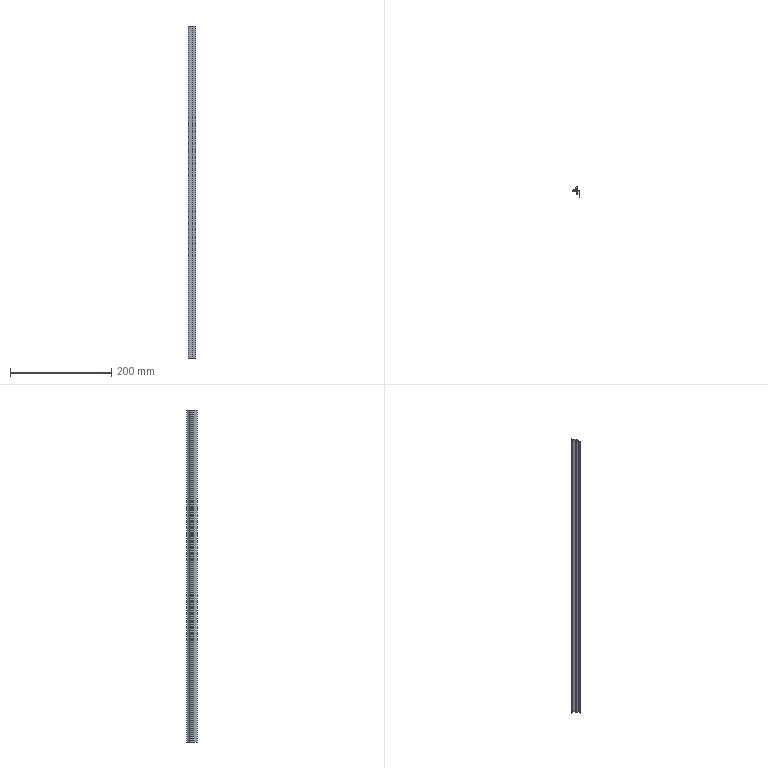Part | SolidWorks | features BaseBody 1, ICE 1, MoveFace 1 | 1 solid | 27 faces | box 14 x 20.3 x 657 mm | volume 33452 mm3 | plane 20 | cylinder 7 | commonest cylinder face diameters 0.387 x2 0.8 x2 0.4 x1 20 x1 22 x1
STEP:
#1=CARTESIAN_POINT('',(-5.304,-0.625,200.));
#2=VERTEX_POINT('',#1);
#3=CARTESIAN_POINT('',(-5.449,-0.8125,200.));
#4=VERTEX_POINT('',#3);
#5=CARTESIAN_POINT('',(-5.255,-0.8125,200.));
#6=DIRECTION('',(0.,0.,1.));
#7=DIRECTION('',(-1.,0.,0.));
#8=AXIS2_PLACEMENT_3D('',#5,#6,#7);
#9=CIRCLE('',#8,0.1937);
#10=EDGE_CURVE('',#2,#4,#9,.T.);
#11=ORIENTED_EDGE('',*,*,#10,.T.);
#12=CARTESIAN_POINT('',(-5.449,-0.8125,-457.));
#13=VERTEX_POINT('',#12);
#14=CARTESIAN_POINT('',(-5.449,-0.8125,230.));
#15=DIRECTION('',(0.,0.,-1.));
#16=VECTOR('',#15,1000.);
#17=LINE('',#14,#16);
#18=EDGE_CURVE('',#4,#13,#17,.T.);
#19=ORIENTED_EDGE('',*,*,#18,.T.);
#20=CARTESIAN_POINT('',(-5.304,-0.625,-457.));
#21=VERTEX_POINT('',#20);
#22=CARTESIAN_POINT('',(-5.255,-0.8125,-457.));
#23=DIRECTION('',(0.,0.,-1.));
#24=DIRECTION('',(1.,0.,0.));
#25=AXIS2_PLACEMENT_3D('',#22,#23,#24);
#26=CIRCLE('',#25,0.1937);
#27=EDGE_CURVE('',#13,#21,#26,.T.);
#28=ORIENTED_EDGE('',*,*,#27,.T.);
#29=CARTESIAN_POINT('',(-5.304,-0.625,230.));
#30=DIRECTION('',(0.,0.,-1.));
#31=VECTOR('',#30,1000.);
#32=LINE('',#29,#31);
#33=EDGE_CURVE('',#2,#21,#32,.T.);
#34=ORIENTED_EDGE('',*,*,#33,.F.);
#35=EDGE_LOOP('',(#11,#19,#28,#34));
#36=FACE_OUTER_BOUND('',#35,.T.);
#37=CARTESIAN_POINT('',(-5.255,-0.8125,230.));
#38=DIRECTION('',(0.,0.,-1.));
#39=DIRECTION('',(-1.,0.,0.));
#40=AXIS2_PLACEMENT_3D('',#37,#38,#39);
#41=CYLINDRICAL_SURFACE('',#40,0.1937);
#42=ADVANCED_FACE('',(#36),#41,.F.);
#43=CARTESIAN_POINT('',(5.,-1.,-457.));
#44=VERTEX_POINT('',#43);
#45=CARTESIAN_POINT('',(5.,-14.3,-457.));
#46=VERTEX_POINT('',#45);
#47=CARTESIAN_POINT('',(5.,29.623,-457.));
#48=DIRECTION('',(0.,-1.,0.));
#49=VECTOR('',#48,1000.);
#50=LINE('',#47,#49);
#51=EDGE_CURVE('',#44,#46,#50,.T.);
#52=ORIENTED_EDGE('',*,*,#51,.F.);
#53=CARTESIAN_POINT('',(5.,-1.,200.));
#54=VERTEX_POINT('',#53);
#55=CARTESIAN_POINT('',(5.,-1.,230.));
#56=DIRECTION('',(0.,0.,-1.));
#57=VECTOR('',#56,1000.);
#58=LINE('',#55,#57);
#59=EDGE_CURVE('',#54,#44,#58,.T.);
#60=ORIENTED_EDGE('',*,*,#59,.F.);
#61=CARTESIAN_POINT('',(5.,-14.3,200.));
#62=VERTEX_POINT('',#61);
#63=CARTESIAN_POINT('',(5.,-14.3,200.));
#64=DIRECTION('',(0.,1.,0.));
#65=VECTOR('',#64,1000.);
#66=LINE('',#63,#65);
#67=EDGE_CURVE('',#62,#54,#66,.T.);
#68=ORIENTED_EDGE('',*,*,#67,.F.);
#69=CARTESIAN_POINT('',(5.,-14.3,230.));
#70=DIRECTION('',(0.,0.,1.));
#71=VECTOR('',#70,1000.);
#72=LINE('',#69,#71);
#73=EDGE_CURVE('',#46,#62,#72,.T.);
#74=ORIENTED_EDGE('',*,*,#73,.F.);
#75=EDGE_LOOP('',(#52,#60,#68,#74));
#76=FACE_OUTER_BOUND('',#75,.T.);
#77=CARTESIAN_POINT('',(5.,-14.3,230.));
#78=DIRECTION('',(-1.,0.,0.));
#79=DIRECTION('',(0.,0.,1.));
#80=AXIS2_PLACEMENT_3D('',#77,#78,#79);
#81=PLANE('',#80);
#82=ADVANCED_FACE('',(#76),#81,.F.);
#83=CARTESIAN_POINT('',(-9.,-2.,-457.));
#84=VERTEX_POINT('',#83);
#85=CARTESIAN_POINT('',(-9.,-2.,200.));
#86=VERTEX_POINT('',#85);
#87=CARTESIAN_POINT('',(-9.,-2.,230.));
#88=DIRECTION('',(0.,0.,1.));
#89=VECTOR('',#88,1000.);
#90=LINE('',#87,#89);
#91=EDGE_CURVE('',#84,#86,#90,.T.);
#92=ORIENTED_EDGE('',*,*,#91,.F.);
#93=CARTESIAN_POINT('',(0.9,-2.,-457.));
#94=VERTEX_POINT('',#93);
#95=CARTESIAN_POINT('',(5.,-2.,-457.));
#96=DIRECTION('',(-1.,0.,0.));
#97=VECTOR('',#96,1000.);
#98=LINE('',#95,#97);
#99=EDGE_CURVE('',#94,#84,#98,.T.);
#100=ORIENTED_EDGE('',*,*,#99,.F.);
#101=CARTESIAN_POINT('',(0.9,-2.,200.));
#102=VERTEX_POINT('',#101);
#103=CARTESIAN_POINT('',(0.9,-2.,230.));
#104=DIRECTION('',(0.,0.,-1.));
#105=VECTOR('',#104,1000.);
#106=LINE('',#103,#105);
#107=EDGE_CURVE('',#102,#94,#106,.T.);
#108=ORIENTED_EDGE('',*,*,#107,.F.);
#109=CARTESIAN_POINT('',(5.,-2.,200.));
#110=DIRECTION('',(1.,0.,0.));
#111=VECTOR('',#110,1000.);
#112=LINE('',#109,#111);
#113=EDGE_CURVE('',#86,#102,#112,.T.);
#114=ORIENTED_EDGE('',*,*,#113,.F.);
#115=EDGE_LOOP('',(#92,#100,#108,#114));
#116=FACE_OUTER_BOUND('',#115,.T.);
#117=CARTESIAN_POINT('',(-9.,-2.,230.));
#118=DIRECTION('',(0.,1.,0.));
#119=DIRECTION('',(0.,0.,1.));
#120=AXIS2_PLACEMENT_3D('',#117,#118,#119);
#121=PLANE('',#120);
#122=ADVANCED_FACE('',(#116),#121,.F.);
#123=CARTESIAN_POINT('',(4.,-6.,200.));
#124=VERTEX_POINT('',#123);
#125=CARTESIAN_POINT('',(4.,-3.,200.));
#126=VERTEX_POINT('',#125);
#127=CARTESIAN_POINT('',(4.,29.623,200.));
#128=DIRECTION('',(0.,1.,0.));
#129=VECTOR('',#128,1000.);
#130=LINE('',#127,#129);
#131=EDGE_CURVE('',#124,#126,#130,.T.);
#132=ORIENTED_EDGE('',*,*,#131,.F.);
#133=CARTESIAN_POINT('',(1.,-6.,200.));
#134=VERTEX_POINT('',#133);
#135=CARTESIAN_POINT('',(5.,-6.,200.));
#136=DIRECTION('',(1.,0.,0.));
#137=VECTOR('',#136,1000.);
#138=LINE('',#135,#137);
#139=EDGE_CURVE('',#134,#124,#138,.T.);
#140=ORIENTED_EDGE('',*,*,#139,.F.);
#141=CARTESIAN_POINT('',(1.,-6.7,200.));
#142=VERTEX_POINT('',#141);
#143=CARTESIAN_POINT('',(1.,-6.,200.));
#144=DIRECTION('',(0.,-1.,0.));
#145=VECTOR('',#144,1000.);
#146=LINE('',#143,#145);
#147=EDGE_CURVE('',#134,#142,#146,.T.);
#148=ORIENTED_EDGE('',*,*,#147,.T.);
#149=CARTESIAN_POINT('',(-1.7,-6.7,200.));
#150=VERTEX_POINT('',#149);
#151=CARTESIAN_POINT('',(5.,-6.7,200.));
#152=DIRECTION('',(1.,0.,0.));
#153=VECTOR('',#152,1000.);
#154=LINE('',#151,#153);
#155=EDGE_CURVE('',#150,#142,#154,.T.);
#156=ORIENTED_EDGE('',*,*,#155,.F.);
#157=CARTESIAN_POINT('',(-1.7,-7.7,200.));
#158=VERTEX_POINT('',#157);
#159=CARTESIAN_POINT('',(-1.7,-6.7,200.));
#160=DIRECTION('',(0.,-1.,0.));
#161=VECTOR('',#160,1000.);
#162=LINE('',#159,#161);
#163=EDGE_CURVE('',#150,#158,#162,.T.);
#164=ORIENTED_EDGE('',*,*,#163,.T.);
#165=CARTESIAN_POINT('',(4.,-7.7,200.));
#166=VERTEX_POINT('',#165);
#167=CARTESIAN_POINT('',(5.,-7.7,200.));
#168=DIRECTION('',(-1.,0.,0.));
#169=VECTOR('',#168,1000.);
#170=LINE('',#167,#169);
#171=EDGE_CURVE('',#166,#158,#170,.T.);
#172=ORIENTED_EDGE('',*,*,#171,.F.);
#173=CARTESIAN_POINT('',(4.,-14.3,200.));
#174=VERTEX_POINT('',#173);
#175=CARTESIAN_POINT('',(4.,29.623,200.));
#176=DIRECTION('',(0.,1.,0.));
#177=VECTOR('',#176,1000.);
#178=LINE('',#175,#177);
#179=EDGE_CURVE('',#174,#166,#178,.T.);
#180=ORIENTED_EDGE('',*,*,#179,.F.);
#181=CARTESIAN_POINT('',(5.,-14.3,200.));
#182=DIRECTION('',(-1.,0.,0.));
#183=VECTOR('',#182,1000.);
#184=LINE('',#181,#183);
#185=EDGE_CURVE('',#62,#174,#184,.T.);
#186=ORIENTED_EDGE('',*,*,#185,.F.);
#187=ORIENTED_EDGE('',*,*,#67,.T.);
#188=CARTESIAN_POINT('',(-5.207,-1.,200.));
#189=VERTEX_POINT('',#188);
#190=CARTESIAN_POINT('',(5.,-1.,200.));
#191=DIRECTION('',(1.,0.,0.));
#192=VECTOR('',#191,1000.);
#193=LINE('',#190,#192);
#194=EDGE_CURVE('',#189,#54,#193,.T.);
#195=ORIENTED_EDGE('',*,*,#194,.F.);
#196=CARTESIAN_POINT('',(-5.255,-0.8125,200.));
#197=DIRECTION('',(0.,0.,1.));
#198=DIRECTION('',(-1.,0.,0.));
#199=AXIS2_PLACEMENT_3D('',#196,#197,#198);
#200=CIRCLE('',#199,0.1937);
#201=EDGE_CURVE('',#4,#189,#200,.T.);
#202=ORIENTED_EDGE('',*,*,#201,.F.);
#203=ORIENTED_EDGE('',*,*,#10,.F.);
#204=CARTESIAN_POINT('',(-1.368,3.063,200.));
#205=VERTEX_POINT('',#204);
#206=CARTESIAN_POINT('',(-10.628,9.,200.));
#207=DIRECTION('',(0.,0.,1.));
#208=DIRECTION('',(-1.,0.,0.));
#209=AXIS2_PLACEMENT_3D('',#206,#207,#208);
#210=CIRCLE('',#209,11.);
#211=EDGE_CURVE('',#2,#205,#210,.T.);
#212=ORIENTED_EDGE('',*,*,#211,.T.);
#213=CARTESIAN_POINT('',(-1.,2.955,200.));
#214=VERTEX_POINT('',#213);
#215=CARTESIAN_POINT('',(-1.2,2.955,200.));
#216=DIRECTION('',(0.,0.,1.));
#217=DIRECTION('',(-1.,0.,0.));
#218=AXIS2_PLACEMENT_3D('',#215,#216,#217);
#219=CIRCLE('',#218,0.2);
#220=EDGE_CURVE('',#214,#205,#219,.T.);
#221=ORIENTED_EDGE('',*,*,#220,.F.);
#222=CARTESIAN_POINT('',(-1.,1.5,200.));
#223=VERTEX_POINT('',#222);
#224=CARTESIAN_POINT('',(-1.,2.955,200.));
#225=DIRECTION('',(0.,1.,0.));
#226=VECTOR('',#225,1000.);
#227=LINE('',#224,#226);
#228=EDGE_CURVE('',#223,#214,#227,.T.);
#229=ORIENTED_EDGE('',*,*,#228,.F.);
#230=CARTESIAN_POINT('',(0.,1.5,200.));
#231=VERTEX_POINT('',#230);
#232=CARTESIAN_POINT('',(-1.,1.5,200.));
#233=DIRECTION('',(-1.,0.,0.));
#234=VECTOR('',#233,1000.);
#235=LINE('',#232,#234);
#236=EDGE_CURVE('',#231,#223,#235,.T.);
#237=ORIENTED_EDGE('',*,*,#236,.F.);
#238=CARTESIAN_POINT('',(0.,6.,200.));
#239=VERTEX_POINT('',#238);
#240=CARTESIAN_POINT('',(0.,1.5,200.));
#241=DIRECTION('',(0.,-1.,0.));
#242=VECTOR('',#241,1000.);
#243=LINE('',#240,#242);
#244=EDGE_CURVE('',#239,#231,#243,.T.);
#245=ORIENTED_EDGE('',*,*,#244,.F.);
#246=CARTESIAN_POINT('',(-0.8,6.,200.));
#247=VERTEX_POINT('',#246);
#248=CARTESIAN_POINT('',(0.,6.,200.));
#249=DIRECTION('',(1.,0.,0.));
#250=VECTOR('',#249,1000.);
#251=LINE('',#248,#250);
#252=EDGE_CURVE('',#247,#239,#251,.T.);
#253=ORIENTED_EDGE('',*,*,#252,.F.);
#254=CARTESIAN_POINT('',(-1.178,5.731,200.));
#255=VERTEX_POINT('',#254);
#256=CARTESIAN_POINT('',(-0.8,5.6,200.));
#257=DIRECTION('',(0.,0.,1.));
#258=DIRECTION('',(-1.,0.,0.));
#259=AXIS2_PLACEMENT_3D('',#256,#257,#258);
#260=CIRCLE('',#259,0.4);
#261=EDGE_CURVE('',#247,#255,#260,.T.);
#262=ORIENTED_EDGE('',*,*,#261,.T.);
#263=CARTESIAN_POINT('',(-8.678,-0.8077,200.));
#264=VERTEX_POINT('',#263);
#265=CARTESIAN_POINT('',(-10.628,9.,200.));
#266=DIRECTION('',(0.,0.,1.));
#267=DIRECTION('',(-1.,0.,0.));
#268=AXIS2_PLACEMENT_3D('',#265,#266,#267);
#269=CIRCLE('',#268,10.);
#270=EDGE_CURVE('',#264,#255,#269,.T.);
#271=ORIENTED_EDGE('',*,*,#270,.F.);
#272=CARTESIAN_POINT('',(-9.,-1.2,200.));
#273=VERTEX_POINT('',#272);
#274=CARTESIAN_POINT('',(-8.6,-1.2,200.));
#275=DIRECTION('',(0.,0.,1.));
#276=DIRECTION('',(-1.,0.,0.));
#277=AXIS2_PLACEMENT_3D('',#274,#275,#276);
#278=CIRCLE('',#277,0.4);
#279=EDGE_CURVE('',#264,#273,#278,.T.);
#280=ORIENTED_EDGE('',*,*,#279,.T.);
#281=CARTESIAN_POINT('',(-9.,8.,200.));
#282=DIRECTION('',(0.,-1.,0.));
#283=VECTOR('',#282,1000.);
#284=LINE('',#281,#283);
#285=EDGE_CURVE('',#273,#86,#284,.T.);
#286=ORIENTED_EDGE('',*,*,#285,.T.);
#287=ORIENTED_EDGE('',*,*,#113,.T.);
#288=CARTESIAN_POINT('',(0.9,-3.,200.));
#289=VERTEX_POINT('',#288);
#290=CARTESIAN_POINT('',(0.9,29.623,200.));
#291=DIRECTION('',(0.,1.,0.));
#292=VECTOR('',#291,1000.);
#293=LINE('',#290,#292);
#294=EDGE_CURVE('',#289,#102,#293,.T.);
#295=ORIENTED_EDGE('',*,*,#294,.F.);
#296=CARTESIAN_POINT('',(5.,-3.,200.));
#297=DIRECTION('',(-1.,0.,0.));
#298=VECTOR('',#297,1000.);
#299=LINE('',#296,#298);
#300=EDGE_CURVE('',#126,#289,#299,.T.);
#301=ORIENTED_EDGE('',*,*,#300,.F.);
#302=EDGE_LOOP('',(#132,#140,#148,#156,#164,#172,#180,#186,#187,#195,#202,#203,#212,#221,#229,#237,#245,#253,#262,#271,#280,#286,#287,#295,#301));
#303=FACE_OUTER_BOUND('',#302,.T.);
#304=CARTESIAN_POINT('',(5.,29.623,200.));
#305=DIRECTION('',(0.,0.,-1.));
#306=DIRECTION('',(-1.,0.,0.));
#307=AXIS2_PLACEMENT_3D('',#304,#305,#306);
#308=PLANE('',#307);
#309=ADVANCED_FACE('',(#303),#308,.F.);
#310=ORIENTED_EDGE('',*,*,#185,.T.);
#311=CARTESIAN_POINT('',(4.,-14.3,-457.));
#312=VERTEX_POINT('',#311);
#313=CARTESIAN_POINT('',(4.,-14.3,230.));
#314=DIRECTION('',(0.,0.,1.));
#315=VECTOR('',#314,1000.);
#316=LINE('',#313,#315);
#317=EDGE_CURVE('',#312,#174,#316,.T.);
#318=ORIENTED_EDGE('',*,*,#317,.F.);
#319=CARTESIAN_POINT('',(5.,-14.3,-457.));
#320=DIRECTION('',(-1.,0.,0.));
#321=VECTOR('',#320,1000.);
#322=LINE('',#319,#321);
#323=EDGE_CURVE('',#46,#312,#322,.T.);
#324=ORIENTED_EDGE('',*,*,#323,.F.);
#325=ORIENTED_EDGE('',*,*,#73,.T.);
#326=EDGE_LOOP('',(#310,#318,#324,#325));
#327=FACE_OUTER_BOUND('',#326,.T.);
#328=CARTESIAN_POINT('',(4.,-14.3,230.));
#329=DIRECTION('',(0.,1.,0.));
#330=DIRECTION('',(0.,0.,1.));
#331=AXIS2_PLACEMENT_3D('',#328,#329,#330);
#332=PLANE('',#331);
#333=ADVANCED_FACE('',(#327),#332,.F.);
#334=ORIENTED_EDGE('',*,*,#51,.T.);
#335=ORIENTED_EDGE('',*,*,#323,.T.);
#336=CARTESIAN_POINT('',(4.,-7.7,-457.));
#337=VERTEX_POINT('',#336);
#338=CARTESIAN_POINT('',(4.,-7.7,-457.));
#339=DIRECTION('',(0.,-1.,0.));
#340=VECTOR('',#339,1000.);
#341=LINE('',#338,#340);
#342=EDGE_CURVE('',#337,#312,#341,.T.);
#343=ORIENTED_EDGE('',*,*,#342,.F.);
#344=CARTESIAN_POINT('',(-1.7,-7.7,-457.));
#345=VERTEX_POINT('',#344);
#346=CARTESIAN_POINT('',(-1.7,-7.7,-457.));
#347=DIRECTION('',(1.,0.,0.));
#348=VECTOR('',#347,1000.);
#349=LINE('',#346,#348);
#350=EDGE_CURVE('',#345,#337,#349,.T.);
#351=ORIENTED_EDGE('',*,*,#350,.F.);
#352=CARTESIAN_POINT('',(-1.7,-6.7,-457.));
#353=VERTEX_POINT('',#352);
#354=CARTESIAN_POINT('',(-1.7,29.623,-457.));
#355=DIRECTION('',(0.,1.,0.));
#356=VECTOR('',#355,1000.);
#357=LINE('',#354,#356);
#358=EDGE_CURVE('',#345,#353,#357,.T.);
#359=ORIENTED_EDGE('',*,*,#358,.T.);
#360=CARTESIAN_POINT('',(1.,-6.7,-457.));
#361=VERTEX_POINT('',#360);
#362=CARTESIAN_POINT('',(1.,-6.7,-457.));
#363=DIRECTION('',(-1.,0.,0.));
#364=VECTOR('',#363,1000.);
#365=LINE('',#362,#364);
#366=EDGE_CURVE('',#361,#353,#365,.T.);
#367=ORIENTED_EDGE('',*,*,#366,.F.);
#368=CARTESIAN_POINT('',(1.,-6.,-457.));
#369=VERTEX_POINT('',#368);
#370=CARTESIAN_POINT('',(1.,29.623,-457.));
#371=DIRECTION('',(0.,1.,0.));
#372=VECTOR('',#371,1000.);
#373=LINE('',#370,#372);
#374=EDGE_CURVE('',#361,#369,#373,.T.);
#375=ORIENTED_EDGE('',*,*,#374,.T.);
#376=CARTESIAN_POINT('',(4.,-6.,-457.));
#377=VERTEX_POINT('',#376);
#378=CARTESIAN_POINT('',(4.,-6.,-457.));
#379=DIRECTION('',(-1.,0.,0.));
#380=VECTOR('',#379,1000.);
#381=LINE('',#378,#380);
#382=EDGE_CURVE('',#377,#369,#381,.T.);
#383=ORIENTED_EDGE('',*,*,#382,.F.);
#384=CARTESIAN_POINT('',(4.,-3.,-457.));
#385=VERTEX_POINT('',#384);
#386=CARTESIAN_POINT('',(4.,-3.,-457.));
#387=DIRECTION('',(0.,-1.,0.));
#388=VECTOR('',#387,1000.);
#389=LINE('',#386,#388);
#390=EDGE_CURVE('',#385,#377,#389,.T.);
#391=ORIENTED_EDGE('',*,*,#390,.F.);
#392=CARTESIAN_POINT('',(0.9,-3.,-457.));
#393=VERTEX_POINT('',#392);
#394=CARTESIAN_POINT('',(0.9,-3.,-457.));
#395=DIRECTION('',(1.,0.,0.));
#396=VECTOR('',#395,1000.);
#397=LINE('',#394,#396);
#398=EDGE_CURVE('',#393,#385,#397,.T.);
#399=ORIENTED_EDGE('',*,*,#398,.F.);
#400=CARTESIAN_POINT('',(0.9,-2.,-457.));
#401=DIRECTION('',(0.,-1.,0.));
#402=VECTOR('',#401,1000.);
#403=LINE('',#400,#402);
#404=EDGE_CURVE('',#94,#393,#403,.T.);
#405=ORIENTED_EDGE('',*,*,#404,.F.);
#406=ORIENTED_EDGE('',*,*,#99,.T.);
#407=CARTESIAN_POINT('',(-9.,-1.2,-457.));
#408=VERTEX_POINT('',#407);
#409=CARTESIAN_POINT('',(-9.,-1.2,-457.));
#410=DIRECTION('',(0.,-1.,0.));
#411=VECTOR('',#410,1000.);
#412=LINE('',#409,#411);
#413=EDGE_CURVE('',#408,#84,#412,.T.);
#414=ORIENTED_EDGE('',*,*,#413,.F.);
#415=CARTESIAN_POINT('',(-8.678,-0.8077,-457.));
#416=VERTEX_POINT('',#415);
#417=CARTESIAN_POINT('',(-8.6,-1.2,-457.));
#418=DIRECTION('',(0.,0.,-1.));
#419=DIRECTION('',(1.,0.,0.));
#420=AXIS2_PLACEMENT_3D('',#417,#418,#419);
#421=CIRCLE('',#420,0.4);
#422=EDGE_CURVE('',#408,#416,#421,.T.);
#423=ORIENTED_EDGE('',*,*,#422,.T.);
#424=CARTESIAN_POINT('',(-1.178,5.731,-457.));
#425=VERTEX_POINT('',#424);
#426=CARTESIAN_POINT('',(-10.628,9.,-457.));
#427=DIRECTION('',(0.,0.,-1.));
#428=DIRECTION('',(1.,0.,0.));
#429=AXIS2_PLACEMENT_3D('',#426,#427,#428);
#430=CIRCLE('',#429,10.);
#431=EDGE_CURVE('',#425,#416,#430,.T.);
#432=ORIENTED_EDGE('',*,*,#431,.F.);
#433=CARTESIAN_POINT('',(-0.8,6.,-457.));
#434=VERTEX_POINT('',#433);
#435=CARTESIAN_POINT('',(-0.8,5.6,-457.));
#436=DIRECTION('',(0.,0.,-1.));
#437=DIRECTION('',(1.,0.,0.));
#438=AXIS2_PLACEMENT_3D('',#435,#436,#437);
#439=CIRCLE('',#438,0.4);
#440=EDGE_CURVE('',#425,#434,#439,.T.);
#441=ORIENTED_EDGE('',*,*,#440,.T.);
#442=CARTESIAN_POINT('',(0.,6.,-457.));
#443=VERTEX_POINT('',#442);
#444=CARTESIAN_POINT('',(0.,6.,-457.));
#445=DIRECTION('',(-1.,0.,0.));
#446=VECTOR('',#445,1000.);
#447=LINE('',#444,#446);
#448=EDGE_CURVE('',#443,#434,#447,.T.);
#449=ORIENTED_EDGE('',*,*,#448,.F.);
#450=CARTESIAN_POINT('',(0.,1.5,-457.));
#451=VERTEX_POINT('',#450);
#452=CARTESIAN_POINT('',(0.,1.5,-457.));
#453=DIRECTION('',(0.,1.,0.));
#454=VECTOR('',#453,1000.);
#455=LINE('',#452,#454);
#456=EDGE_CURVE('',#451,#443,#455,.T.);
#457=ORIENTED_EDGE('',*,*,#456,.F.);
#458=CARTESIAN_POINT('',(-1.,1.5,-457.));
#459=VERTEX_POINT('',#458);
#460=CARTESIAN_POINT('',(-1.,1.5,-457.));
#461=DIRECTION('',(1.,0.,0.));
#462=VECTOR('',#461,1000.);
#463=LINE('',#460,#462);
#464=EDGE_CURVE('',#459,#451,#463,.T.);
#465=ORIENTED_EDGE('',*,*,#464,.F.);
#466=CARTESIAN_POINT('',(-1.,2.955,-457.));
#467=VERTEX_POINT('',#466);
#468=CARTESIAN_POINT('',(-1.,2.955,-457.));
#469=DIRECTION('',(0.,-1.,0.));
#470=VECTOR('',#469,1000.);
#471=LINE('',#468,#470);
#472=EDGE_CURVE('',#467,#459,#471,.T.);
#473=ORIENTED_EDGE('',*,*,#472,.F.);
#474=CARTESIAN_POINT('',(-1.368,3.063,-457.));
#475=VERTEX_POINT('',#474);
#476=CARTESIAN_POINT('',(-1.2,2.955,-457.));
#477=DIRECTION('',(0.,0.,-1.));
#478=DIRECTION('',(1.,0.,0.));
#479=AXIS2_PLACEMENT_3D('',#476,#477,#478);
#480=CIRCLE('',#479,0.2);
#481=EDGE_CURVE('',#475,#467,#480,.T.);
#482=ORIENTED_EDGE('',*,*,#481,.F.);
#483=CARTESIAN_POINT('',(-10.628,9.,-457.));
#484=DIRECTION('',(0.,0.,-1.));
#485=DIRECTION('',(1.,0.,0.));
#486=AXIS2_PLACEMENT_3D('',#483,#484,#485);
#487=CIRCLE('',#486,11.);
#488=EDGE_CURVE('',#475,#21,#487,.T.);
#489=ORIENTED_EDGE('',*,*,#488,.T.);
#490=ORIENTED_EDGE('',*,*,#27,.F.);
#491=CARTESIAN_POINT('',(-5.207,-1.,-457.));
#492=VERTEX_POINT('',#491);
#493=CARTESIAN_POINT('',(-5.255,-0.8125,-457.));
#494=DIRECTION('',(0.,0.,-1.));
#495=DIRECTION('',(1.,0.,0.));
#496=AXIS2_PLACEMENT_3D('',#493,#494,#495);
#497=CIRCLE('',#496,0.1937);
#498=EDGE_CURVE('',#492,#13,#497,.T.);
#499=ORIENTED_EDGE('',*,*,#498,.F.);
#500=CARTESIAN_POINT('',(5.,-1.,-457.));
#501=DIRECTION('',(-1.,0.,0.));
#502=VECTOR('',#501,1000.);
#503=LINE('',#500,#502);
#504=EDGE_CURVE('',#44,#492,#503,.T.);
#505=ORIENTED_EDGE('',*,*,#504,.F.);
#506=EDGE_LOOP('',(#334,#335,#343,#351,#359,#367,#375,#383,#391,#399,#405,#406,#414,#423,#432,#441,#449,#457,#465,#473,#482,#489,#490,#499,#505));
#507=FACE_OUTER_BOUND('',#506,.T.);
#508=CARTESIAN_POINT('',(5.,29.623,-457.));
#509=DIRECTION('',(0.,0.,1.));
#510=DIRECTION('',(1.,0.,0.));
#511=AXIS2_PLACEMENT_3D('',#508,#509,#510);
#512=PLANE('',#511);
#513=ADVANCED_FACE('',(#507),#512,.F.);
#514=ORIENTED_EDGE('',*,*,#59,.T.);
#515=ORIENTED_EDGE('',*,*,#504,.T.);
#516=CARTESIAN_POINT('',(-5.207,-1.,230.));
#517=DIRECTION('',(0.,0.,-1.));
#518=VECTOR('',#517,1000.);
#519=LINE('',#516,#518);
#520=EDGE_CURVE('',#189,#492,#519,.T.);
#521=ORIENTED_EDGE('',*,*,#520,.F.);
#522=ORIENTED_EDGE('',*,*,#194,.T.);
#523=EDGE_LOOP('',(#514,#515,#521,#522));
#524=FACE_OUTER_BOUND('',#523,.T.);
#525=CARTESIAN_POINT('',(5.,-1.,230.));
#526=DIRECTION('',(0.,-1.,0.));
#527=DIRECTION('',(0.,0.,-1.));
#528=AXIS2_PLACEMENT_3D('',#525,#526,#527);
#529=PLANE('',#528);
#530=ADVANCED_FACE('',(#524),#529,.F.);
#531=CARTESIAN_POINT('',(-9.,-1.2,230.));
#532=DIRECTION('',(0.,0.,1.));
#533=VECTOR('',#532,1000.);
#534=LINE('',#531,#533);
#535=EDGE_CURVE('',#408,#273,#534,.T.);
#536=ORIENTED_EDGE('',*,*,#535,.F.);
#537=ORIENTED_EDGE('',*,*,#413,.T.);
#538=ORIENTED_EDGE('',*,*,#91,.T.);
#539=ORIENTED_EDGE('',*,*,#285,.F.);
#540=EDGE_LOOP('',(#536,#537,#538,#539));
#541=FACE_OUTER_BOUND('',#540,.T.);
#542=CARTESIAN_POINT('',(-9.,-1.2,230.));
#543=DIRECTION('',(1.,0.,0.));
#544=DIRECTION('',(0.,0.,-1.));
#545=AXIS2_PLACEMENT_3D('',#542,#543,#544);
#546=PLANE('',#545);
#547=ADVANCED_FACE('',(#541),#546,.F.);
#548=ORIENTED_EDGE('',*,*,#294,.T.);
#549=ORIENTED_EDGE('',*,*,#107,.T.);
#550=ORIENTED_EDGE('',*,*,#404,.T.);
#551=CARTESIAN_POINT('',(0.9,-3.,230.));
#552=DIRECTION('',(0.,0.,-1.));
#553=VECTOR('',#552,1000.);
#554=LINE('',#551,#553);
#555=EDGE_CURVE('',#289,#393,#554,.T.);
#556=ORIENTED_EDGE('',*,*,#555,.F.);
#557=EDGE_LOOP('',(#548,#549,#550,#556));
#558=FACE_OUTER_BOUND('',#557,.T.);
#559=CARTESIAN_POINT('',(0.9,-2.,230.));
#560=DIRECTION('',(1.,0.,0.));
#561=DIRECTION('',(0.,0.,-1.));
#562=AXIS2_PLACEMENT_3D('',#559,#560,#561);
#563=PLANE('',#562);
#564=ADVANCED_FACE('',(#558),#563,.F.);
#565=ORIENTED_EDGE('',*,*,#300,.T.);
#566=ORIENTED_EDGE('',*,*,#555,.T.);
#567=ORIENTED_EDGE('',*,*,#398,.T.);
#568=CARTESIAN_POINT('',(4.,-3.,230.));
#569=DIRECTION('',(0.,0.,-1.));
#570=VECTOR('',#569,1000.);
#571=LINE('',#568,#570);
#572=EDGE_CURVE('',#126,#385,#571,.T.);
#573=ORIENTED_EDGE('',*,*,#572,.F.);
#574=EDGE_LOOP('',(#565,#566,#567,#573));
#575=FACE_OUTER_BOUND('',#574,.T.);
#576=CARTESIAN_POINT('',(0.9,-3.,230.));
#577=DIRECTION('',(0.,1.,0.));
#578=DIRECTION('',(0.,0.,1.));
#579=AXIS2_PLACEMENT_3D('',#576,#577,#578);
#580=PLANE('',#579);
#581=ADVANCED_FACE('',(#575),#580,.F.);
#582=ORIENTED_EDGE('',*,*,#131,.T.);
#583=ORIENTED_EDGE('',*,*,#572,.T.);
#584=ORIENTED_EDGE('',*,*,#390,.T.);
#585=CARTESIAN_POINT('',(4.,-6.,230.));
#586=DIRECTION('',(0.,0.,-1.));
#587=VECTOR('',#586,1000.);
#588=LINE('',#585,#587);
#589=EDGE_CURVE('',#124,#377,#588,.T.);
#590=ORIENTED_EDGE('',*,*,#589,.F.);
#591=EDGE_LOOP('',(#582,#583,#584,#590));
#592=FACE_OUTER_BOUND('',#591,.T.);
#593=CARTESIAN_POINT('',(4.,-3.,230.));
#594=DIRECTION('',(1.,0.,0.));
#595=DIRECTION('',(0.,0.,-1.));
#596=AXIS2_PLACEMENT_3D('',#593,#594,#595);
#597=PLANE('',#596);
#598=ADVANCED_FACE('',(#592),#597,.F.);
#599=ORIENTED_EDGE('',*,*,#139,.T.);
#600=ORIENTED_EDGE('',*,*,#589,.T.);
#601=ORIENTED_EDGE('',*,*,#382,.T.);
#602=CARTESIAN_POINT('',(1.,-6.,230.));
#603=DIRECTION('',(0.,0.,-1.));
#604=VECTOR('',#603,1000.);
#605=LINE('',#602,#604);
#606=EDGE_CURVE('',#134,#369,#605,.T.);
#607=ORIENTED_EDGE('',*,*,#606,.F.);
#608=EDGE_LOOP('',(#599,#600,#601,#607));
#609=FACE_OUTER_BOUND('',#608,.T.);
#610=CARTESIAN_POINT('',(4.,-6.,230.));
#611=DIRECTION('',(0.,-1.,0.));
#612=DIRECTION('',(0.,0.,-1.));
#613=AXIS2_PLACEMENT_3D('',#610,#611,#612);
#614=PLANE('',#613);
#615=ADVANCED_FACE('',(#609),#614,.F.);
#616=ORIENTED_EDGE('',*,*,#155,.T.);
#617=CARTESIAN_POINT('',(1.,-6.7,230.));
#618=DIRECTION('',(0.,0.,1.));
#619=VECTOR('',#618,1000.);
#620=LINE('',#617,#619);
#621=EDGE_CURVE('',#361,#142,#620,.T.);
#622=ORIENTED_EDGE('',*,*,#621,.F.);
#623=ORIENTED_EDGE('',*,*,#366,.T.);
#624=CARTESIAN_POINT('',(-1.7,-6.7,230.));
#625=DIRECTION('',(0.,0.,-1.));
#626=VECTOR('',#625,1000.);
#627=LINE('',#624,#626);
#628=EDGE_CURVE('',#150,#353,#627,.T.);
#629=ORIENTED_EDGE('',*,*,#628,.F.);
#630=EDGE_LOOP('',(#616,#622,#623,#629));
#631=FACE_OUTER_BOUND('',#630,.T.);
#632=CARTESIAN_POINT('',(1.,-6.7,230.));
#633=DIRECTION('',(0.,-1.,0.));
#634=DIRECTION('',(0.,0.,-1.));
#635=AXIS2_PLACEMENT_3D('',#632,#633,#634);
#636=PLANE('',#635);
#637=ADVANCED_FACE('',(#631),#636,.F.);
#638=ORIENTED_EDGE('',*,*,#171,.T.);
#639=CARTESIAN_POINT('',(-1.7,-7.7,230.));
#640=DIRECTION('',(0.,0.,1.));
#641=VECTOR('',#640,1000.);
#642=LINE('',#639,#641);
#643=EDGE_CURVE('',#345,#158,#642,.T.);
#644=ORIENTED_EDGE('',*,*,#643,.F.);
#645=ORIENTED_EDGE('',*,*,#350,.T.);
#646=CARTESIAN_POINT('',(4.,-7.7,230.));
#647=DIRECTION('',(0.,0.,-1.));
#648=VECTOR('',#647,1000.);
#649=LINE('',#646,#648);
#650=EDGE_CURVE('',#166,#337,#649,.T.);
#651=ORIENTED_EDGE('',*,*,#650,.F.);
#652=EDGE_LOOP('',(#638,#644,#645,#651));
#653=FACE_OUTER_BOUND('',#652,.T.);
#654=CARTESIAN_POINT('',(-1.7,-7.7,230.));
#655=DIRECTION('',(0.,1.,0.));
#656=DIRECTION('',(0.,0.,1.));
#657=AXIS2_PLACEMENT_3D('',#654,#655,#656);
#658=PLANE('',#657);
#659=ADVANCED_FACE('',(#653),#658,.F.);
#660=ORIENTED_EDGE('',*,*,#179,.T.);
#661=ORIENTED_EDGE('',*,*,#650,.T.);
#662=ORIENTED_EDGE('',*,*,#342,.T.);
#663=ORIENTED_EDGE('',*,*,#317,.T.);
#664=EDGE_LOOP('',(#660,#661,#662,#663));
#665=FACE_OUTER_BOUND('',#664,.T.);
#666=CARTESIAN_POINT('',(4.,-7.7,230.));
#667=DIRECTION('',(1.,0.,0.));
#668=DIRECTION('',(0.,0.,-1.));
#669=AXIS2_PLACEMENT_3D('',#666,#667,#668);
#670=PLANE('',#669);
#671=ADVANCED_FACE('',(#665),#670,.F.);
#672=ORIENTED_EDGE('',*,*,#18,.F.);
#673=ORIENTED_EDGE('',*,*,#201,.T.);
#674=ORIENTED_EDGE('',*,*,#520,.T.);
#675=ORIENTED_EDGE('',*,*,#498,.T.);
#676=EDGE_LOOP('',(#672,#673,#674,#675));
#677=FACE_OUTER_BOUND('',#676,.T.);
#678=CARTESIAN_POINT('',(-5.255,-0.8125,230.));
#679=DIRECTION('',(0.,0.,-1.));
#680=DIRECTION('',(-1.,0.,0.));
#681=AXIS2_PLACEMENT_3D('',#678,#679,#680);
#682=CYLINDRICAL_SURFACE('',#681,0.1937);
#683=ADVANCED_FACE('',(#677),#682,.F.);
#684=CARTESIAN_POINT('',(-1.,2.955,230.));
#685=DIRECTION('',(0.,0.,1.));
#686=VECTOR('',#685,1000.);
#687=LINE('',#684,#686);
#688=EDGE_CURVE('',#467,#214,#687,.T.);
#689=ORIENTED_EDGE('',*,*,#688,.F.);
#690=ORIENTED_EDGE('',*,*,#472,.T.);
#691=CARTESIAN_POINT('',(-1.,1.5,230.));
#692=DIRECTION('',(0.,0.,-1.));
#693=VECTOR('',#692,1000.);
#694=LINE('',#691,#693);
#695=EDGE_CURVE('',#223,#459,#694,.T.);
#696=ORIENTED_EDGE('',*,*,#695,.F.);
#697=ORIENTED_EDGE('',*,*,#228,.T.);
#698=EDGE_LOOP('',(#689,#690,#696,#697));
#699=FACE_OUTER_BOUND('',#698,.T.);
#700=CARTESIAN_POINT('',(-1.,2.955,230.));
#701=DIRECTION('',(1.,0.,0.));
#702=DIRECTION('',(0.,0.,-1.));
#703=AXIS2_PLACEMENT_3D('',#700,#701,#702);
#704=PLANE('',#703);
#705=ADVANCED_FACE('',(#699),#704,.F.);
#706=ORIENTED_EDGE('',*,*,#488,.F.);
#707=CARTESIAN_POINT('',(-1.368,3.063,230.));
#708=DIRECTION('',(0.,0.,1.));
#709=VECTOR('',#708,1000.);
#710=LINE('',#707,#709);
#711=EDGE_CURVE('',#475,#205,#710,.T.);
#712=ORIENTED_EDGE('',*,*,#711,.T.);
#713=ORIENTED_EDGE('',*,*,#211,.F.);
#714=ORIENTED_EDGE('',*,*,#33,.T.);
#715=EDGE_LOOP('',(#706,#712,#713,#714));
#716=FACE_OUTER_BOUND('',#715,.T.);
#717=CARTESIAN_POINT('',(-10.628,9.,230.));
#718=DIRECTION('',(0.,0.,-1.));
#719=DIRECTION('',(-1.,0.,0.));
#720=AXIS2_PLACEMENT_3D('',#717,#718,#719);
#721=CYLINDRICAL_SURFACE('',#720,11.);
#722=ADVANCED_FACE('',(#716),#721,.T.);
#723=CARTESIAN_POINT('',(-1.178,5.731,230.));
#724=DIRECTION('',(0.,0.,1.));
#725=VECTOR('',#724,1000.);
#726=LINE('',#723,#725);
#727=EDGE_CURVE('',#425,#255,#726,.T.);
#728=ORIENTED_EDGE('',*,*,#727,.F.);
#729=ORIENTED_EDGE('',*,*,#431,.T.);
#730=CARTESIAN_POINT('',(-8.678,-0.8077,230.));
#731=DIRECTION('',(0.,0.,-1.));
#732=VECTOR('',#731,1000.);
#733=LINE('',#730,#732);
#734=EDGE_CURVE('',#264,#416,#733,.T.);
#735=ORIENTED_EDGE('',*,*,#734,.F.);
#736=ORIENTED_EDGE('',*,*,#270,.T.);
#737=EDGE_LOOP('',(#728,#729,#735,#736));
#738=FACE_OUTER_BOUND('',#737,.T.);
#739=CARTESIAN_POINT('',(-10.628,9.,230.));
#740=DIRECTION('',(0.,0.,-1.));
#741=DIRECTION('',(-1.,0.,0.));
#742=AXIS2_PLACEMENT_3D('',#739,#740,#741);
#743=CYLINDRICAL_SURFACE('',#742,10.);
#744=ADVANCED_FACE('',(#738),#743,.F.);
#745=CARTESIAN_POINT('',(0.,1.5,230.));
#746=DIRECTION('',(0.,0.,1.));
#747=VECTOR('',#746,1000.);
#748=LINE('',#745,#747);
#749=EDGE_CURVE('',#451,#231,#748,.T.);
#750=ORIENTED_EDGE('',*,*,#749,.F.);
#751=ORIENTED_EDGE('',*,*,#456,.T.);
#752=CARTESIAN_POINT('',(0.,6.,230.));
#753=DIRECTION('',(0.,0.,-1.));
#754=VECTOR('',#753,1000.);
#755=LINE('',#752,#754);
#756=EDGE_CURVE('',#239,#443,#755,.T.);
#757=ORIENTED_EDGE('',*,*,#756,.F.);
#758=ORIENTED_EDGE('',*,*,#244,.T.);
#759=EDGE_LOOP('',(#750,#751,#757,#758));
#760=FACE_OUTER_BOUND('',#759,.T.);
#761=CARTESIAN_POINT('',(0.,1.5,230.));
#762=DIRECTION('',(-1.,0.,0.));
#763=DIRECTION('',(0.,0.,1.));
#764=AXIS2_PLACEMENT_3D('',#761,#762,#763);
#765=PLANE('',#764);
#766=ADVANCED_FACE('',(#760),#765,.F.);
#767=ORIENTED_EDGE('',*,*,#422,.F.);
#768=ORIENTED_EDGE('',*,*,#535,.T.);
#769=ORIENTED_EDGE('',*,*,#279,.F.);
#770=ORIENTED_EDGE('',*,*,#734,.T.);
#771=EDGE_LOOP('',(#767,#768,#769,#770));
#772=FACE_OUTER_BOUND('',#771,.T.);
#773=CARTESIAN_POINT('',(-8.6,-1.2,230.));
#774=DIRECTION('',(0.,0.,-1.));
#775=DIRECTION('',(-1.,0.,0.));
#776=AXIS2_PLACEMENT_3D('',#773,#774,#775);
#777=CYLINDRICAL_SURFACE('',#776,0.4);
#778=ADVANCED_FACE('',(#772),#777,.T.);
#779=ORIENTED_EDGE('',*,*,#147,.F.);
#780=ORIENTED_EDGE('',*,*,#606,.T.);
#781=ORIENTED_EDGE('',*,*,#374,.F.);
#782=ORIENTED_EDGE('',*,*,#621,.T.);
#783=EDGE_LOOP('',(#779,#780,#781,#782));
#784=FACE_OUTER_BOUND('',#783,.T.);
#785=CARTESIAN_POINT('',(1.,-6.,230.));
#786=DIRECTION('',(1.,0.,0.));
#787=DIRECTION('',(0.,0.,-1.));
#788=AXIS2_PLACEMENT_3D('',#785,#786,#787);
#789=PLANE('',#788);
#790=ADVANCED_FACE('',(#784),#789,.F.);
#791=ORIENTED_EDGE('',*,*,#163,.F.);
#792=ORIENTED_EDGE('',*,*,#628,.T.);
#793=ORIENTED_EDGE('',*,*,#358,.F.);
#794=ORIENTED_EDGE('',*,*,#643,.T.);
#795=EDGE_LOOP('',(#791,#792,#793,#794));
#796=FACE_OUTER_BOUND('',#795,.T.);
#797=CARTESIAN_POINT('',(-1.7,-6.7,230.));
#798=DIRECTION('',(1.,0.,0.));
#799=DIRECTION('',(0.,0.,-1.));
#800=AXIS2_PLACEMENT_3D('',#797,#798,#799);
#801=PLANE('',#800);
#802=ADVANCED_FACE('',(#796),#801,.F.);
#803=ORIENTED_EDGE('',*,*,#711,.F.);
#804=ORIENTED_EDGE('',*,*,#481,.T.);
#805=ORIENTED_EDGE('',*,*,#688,.T.);
#806=ORIENTED_EDGE('',*,*,#220,.T.);
#807=EDGE_LOOP('',(#803,#804,#805,#806));
#808=FACE_OUTER_BOUND('',#807,.T.);
#809=CARTESIAN_POINT('',(-1.2,2.955,230.));
#810=DIRECTION('',(0.,0.,-1.));
#811=DIRECTION('',(-1.,0.,0.));
#812=AXIS2_PLACEMENT_3D('',#809,#810,#811);
#813=CYLINDRICAL_SURFACE('',#812,0.2);
#814=ADVANCED_FACE('',(#808),#813,.F.);
#815=ORIENTED_EDGE('',*,*,#695,.T.);
#816=ORIENTED_EDGE('',*,*,#464,.T.);
#817=ORIENTED_EDGE('',*,*,#749,.T.);
#818=ORIENTED_EDGE('',*,*,#236,.T.);
#819=EDGE_LOOP('',(#815,#816,#817,#818));
#820=FACE_OUTER_BOUND('',#819,.T.);
#821=CARTESIAN_POINT('',(-1.,1.5,230.));
#822=DIRECTION('',(0.,1.,0.));
#823=DIRECTION('',(0.,0.,1.));
#824=AXIS2_PLACEMENT_3D('',#821,#822,#823);
#825=PLANE('',#824);
#826=ADVANCED_FACE('',(#820),#825,.F.);
#827=ORIENTED_EDGE('',*,*,#440,.F.);
#828=ORIENTED_EDGE('',*,*,#727,.T.);
#829=ORIENTED_EDGE('',*,*,#261,.F.);
#830=CARTESIAN_POINT('',(-0.8,6.,230.));
#831=DIRECTION('',(0.,0.,-1.));
#832=VECTOR('',#831,1000.);
#833=LINE('',#830,#832);
#834=EDGE_CURVE('',#247,#434,#833,.T.);
#835=ORIENTED_EDGE('',*,*,#834,.T.);
#836=EDGE_LOOP('',(#827,#828,#829,#835));
#837=FACE_OUTER_BOUND('',#836,.T.);
#838=CARTESIAN_POINT('',(-0.8,5.6,230.));
#839=DIRECTION('',(0.,0.,-1.));
#840=DIRECTION('',(-1.,0.,0.));
#841=AXIS2_PLACEMENT_3D('',#838,#839,#840);
#842=CYLINDRICAL_SURFACE('',#841,0.4);
#843=ADVANCED_FACE('',(#837),#842,.T.);
#844=ORIENTED_EDGE('',*,*,#756,.T.);
#845=ORIENTED_EDGE('',*,*,#448,.T.);
#846=ORIENTED_EDGE('',*,*,#834,.F.);
#847=ORIENTED_EDGE('',*,*,#252,.T.);
#848=EDGE_LOOP('',(#844,#845,#846,#847));
#849=FACE_OUTER_BOUND('',#848,.T.);
#850=CARTESIAN_POINT('',(0.,6.,230.));
#851=DIRECTION('',(0.,-1.,0.));
#852=DIRECTION('',(0.,0.,-1.));
#853=AXIS2_PLACEMENT_3D('',#850,#851,#852);
#854=PLANE('',#853);
#855=ADVANCED_FACE('',(#849),#854,.F.);
#856=CLOSED_SHELL('',(#42,#82,#122,#309,#333,#513,#530,#547,#564,#581,#598,#615,#637,#659,#671,#683,#705,#722,#744,#766,#778,#790,#802,#814,#826,#843,#855));
#857=MANIFOLD_SOLID_BREP('',#856);
#858=CARTESIAN_POINT('',(0.,0.,0.));
#859=DIRECTION('',(0.,0.,1.));
#860=DIRECTION('',(1.,0.,0.));
#861=AXIS2_PLACEMENT_3D('',#858,#859,#860);
#862=(LENGTH_UNIT()NAMED_UNIT(*)SI_UNIT(.MILLI.,.METRE.));
#863=UNCERTAINTY_MEASURE_WITH_UNIT(LENGTH_MEASURE(0.00001),#862,'','');
#864=(NAMED_UNIT(*)PLANE_ANGLE_UNIT()SI_UNIT($,.RADIAN.));
#865=(NAMED_UNIT(*)SI_UNIT($,.STERADIAN.)SOLID_ANGLE_UNIT());
#866=(GEOMETRIC_REPRESENTATION_CONTEXT(3)GLOBAL_UNCERTAINTY_ASSIGNED_CONTEXT((#863))GLOBAL_UNIT_ASSIGNED_CONTEXT((#862,#864,#865))REPRESENTATION_CONTEXT('',''));
#867=ADVANCED_BREP_SHAPE_REPRESENTATION('',(#857,#861),#866);